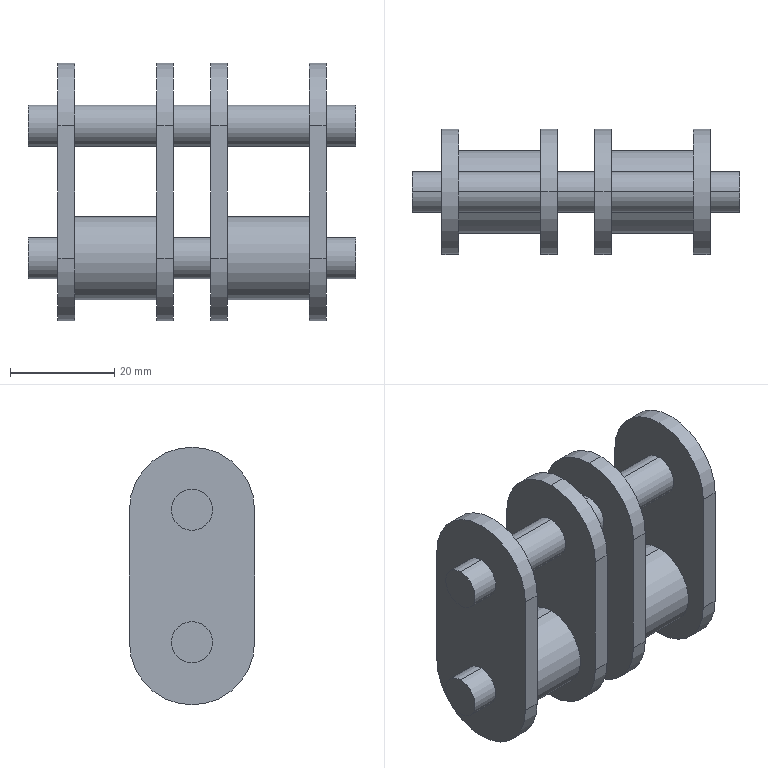Part | SolidWorks | features ICE 6, CombineBodies 1, Extrusion 1, MirrorSolid 1 | 8 solids | 64 faces | box 62.7 x 24 x 49.4 mm | volume 23197 mm3 | cylinder 40 | plane 24 | commonest cylinder face diameters 7.92 x24 24 x12 15.88 x4